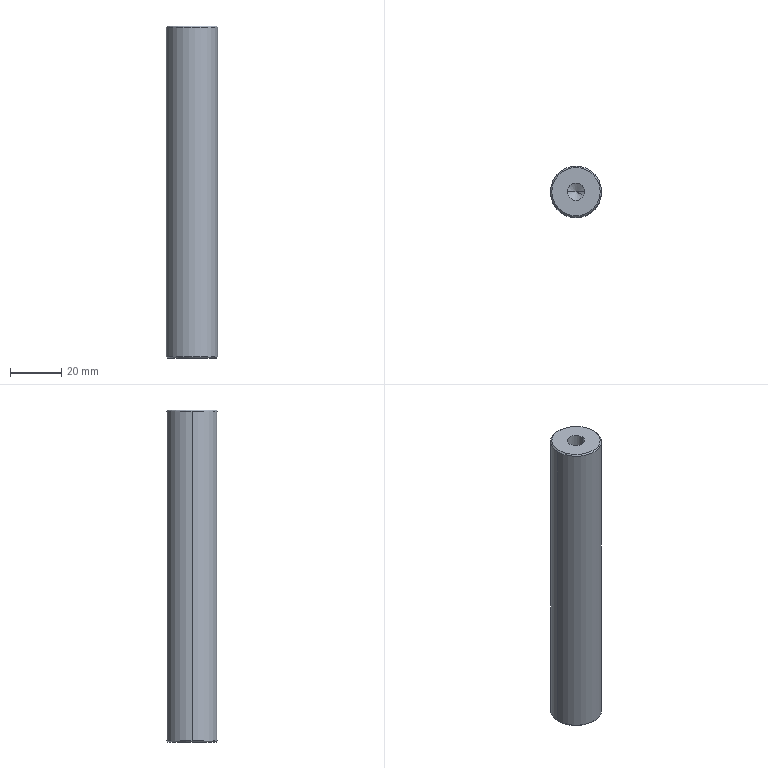Part | SolidWorks | features HoleWzd 2, Chamfer 1, Extrusion 1 | 1 solid | 16 faces | box 20 x 20 x 130 mm | volume 39341 mm3 | cone 8 | cylinder 6 | plane 2 | commonest cylinder face diameters 6.8 x4 20 x2
STEP:
#1=CARTESIAN_POINT('',(9.5,0.,130.));
#2=VERTEX_POINT('',#1);
#3=CARTESIAN_POINT('',(-9.5,0.,130.));
#4=VERTEX_POINT('',#3);
#5=CARTESIAN_POINT('',(0.,0.,130.));
#6=DIRECTION('',(0.,0.,1.));
#7=DIRECTION('',(1.,0.,0.));
#8=AXIS2_PLACEMENT_3D('',#5,#6,#7);
#9=CIRCLE('',#8,9.5);
#10=EDGE_CURVE('',#2,#4,#9,.T.);
#11=ORIENTED_EDGE('',*,*,#10,.F.);
#12=CARTESIAN_POINT('',(10.,0.,129.5));
#13=VERTEX_POINT('',#12);
#14=CARTESIAN_POINT('',(9.5,0.,130.));
#15=DIRECTION('',(0.7071,0.,-0.7071));
#16=VECTOR('',#15,1000.);
#17=LINE('',#14,#16);
#18=EDGE_CURVE('',#2,#13,#17,.T.);
#19=ORIENTED_EDGE('',*,*,#18,.T.);
#20=CARTESIAN_POINT('',(-10.,0.,129.5));
#21=VERTEX_POINT('',#20);
#22=CARTESIAN_POINT('',(0.,0.,129.5));
#23=DIRECTION('',(0.,0.,-1.));
#24=DIRECTION('',(1.,0.,0.));
#25=AXIS2_PLACEMENT_3D('',#22,#23,#24);
#26=CIRCLE('',#25,10.);
#27=EDGE_CURVE('',#21,#13,#26,.T.);
#28=ORIENTED_EDGE('',*,*,#27,.F.);
#29=CARTESIAN_POINT('',(-9.5,0.,130.));
#30=DIRECTION('',(-0.7071,0.,-0.7071));
#31=VECTOR('',#30,1000.);
#32=LINE('',#29,#31);
#33=EDGE_CURVE('',#4,#21,#32,.T.);
#34=ORIENTED_EDGE('',*,*,#33,.F.);
#35=EDGE_LOOP('',(#11,#19,#28,#34));
#36=FACE_OUTER_BOUND('',#35,.T.);
#37=CARTESIAN_POINT('',(0.,0.,130.));
#38=DIRECTION('',(0.,0.,-1.));
#39=DIRECTION('',(-1.,0.,0.));
#40=AXIS2_PLACEMENT_3D('',#37,#38,#39);
#41=CONICAL_SURFACE('',#40,9.5,0.7854);
#42=ADVANCED_FACE('',(#36),#41,.T.);
#43=CARTESIAN_POINT('',(-9.5,0.,0.));
#44=VERTEX_POINT('',#43);
#45=CARTESIAN_POINT('',(9.5,0.,0.));
#46=VERTEX_POINT('',#45);
#47=CARTESIAN_POINT('',(0.,0.,0.));
#48=DIRECTION('',(0.,0.,-1.));
#49=DIRECTION('',(1.,0.,0.));
#50=AXIS2_PLACEMENT_3D('',#47,#48,#49);
#51=CIRCLE('',#50,9.5);
#52=EDGE_CURVE('',#44,#46,#51,.T.);
#53=ORIENTED_EDGE('',*,*,#52,.F.);
#54=CARTESIAN_POINT('',(-10.,0.,0.5));
#55=VERTEX_POINT('',#54);
#56=CARTESIAN_POINT('',(-10.,0.,0.5));
#57=DIRECTION('',(-0.7071,0.,0.7071));
#58=VECTOR('',#57,1000.);
#59=LINE('',#56,#58);
#60=EDGE_CURVE('',#44,#55,#59,.T.);
#61=ORIENTED_EDGE('',*,*,#60,.T.);
#62=CARTESIAN_POINT('',(10.,0.,0.5));
#63=VERTEX_POINT('',#62);
#64=CARTESIAN_POINT('',(0.,0.,0.5));
#65=DIRECTION('',(0.,0.,1.));
#66=DIRECTION('',(1.,0.,0.));
#67=AXIS2_PLACEMENT_3D('',#64,#65,#66);
#68=CIRCLE('',#67,10.);
#69=EDGE_CURVE('',#63,#55,#68,.T.);
#70=ORIENTED_EDGE('',*,*,#69,.F.);
#71=CARTESIAN_POINT('',(10.,0.,0.5));
#72=DIRECTION('',(0.7071,0.,0.7071));
#73=VECTOR('',#72,1000.);
#74=LINE('',#71,#73);
#75=EDGE_CURVE('',#46,#63,#74,.T.);
#76=ORIENTED_EDGE('',*,*,#75,.F.);
#77=EDGE_LOOP('',(#53,#61,#70,#76));
#78=FACE_OUTER_BOUND('',#77,.T.);
#79=CARTESIAN_POINT('',(0.,0.,0.5));
#80=DIRECTION('',(0.,0.,1.));
#81=DIRECTION('',(1.,0.,0.));
#82=AXIS2_PLACEMENT_3D('',#79,#80,#81);
#83=CONICAL_SURFACE('',#82,10.,0.7854);
#84=ADVANCED_FACE('',(#78),#83,.T.);
#85=CARTESIAN_POINT('',(-3.4,0.,110.25));
#86=VERTEX_POINT('',#85);
#87=CARTESIAN_POINT('',(3.4,0.,110.25));
#88=VERTEX_POINT('',#87);
#89=CARTESIAN_POINT('',(0.,0.,110.25));
#90=DIRECTION('',(0.,0.,1.));
#91=DIRECTION('',(1.,0.,0.));
#92=AXIS2_PLACEMENT_3D('',#89,#90,#91);
#93=CIRCLE('',#92,3.4);
#94=EDGE_CURVE('',#86,#88,#93,.T.);
#95=ORIENTED_EDGE('',*,*,#94,.F.);
#96=CARTESIAN_POINT('',(-3.4,0.,130.));
#97=VERTEX_POINT('',#96);
#98=CARTESIAN_POINT('',(-3.4,0.,130.));
#99=DIRECTION('',(0.,0.,1.));
#100=VECTOR('',#99,1000.);
#101=LINE('',#98,#100);
#102=EDGE_CURVE('',#86,#97,#101,.T.);
#103=ORIENTED_EDGE('',*,*,#102,.T.);
#104=CARTESIAN_POINT('',(3.4,0.,130.));
#105=VERTEX_POINT('',#104);
#106=CARTESIAN_POINT('',(0.,0.,130.));
#107=DIRECTION('',(0.,0.,1.));
#108=DIRECTION('',(1.,0.,0.));
#109=AXIS2_PLACEMENT_3D('',#106,#107,#108);
#110=CIRCLE('',#109,3.4);
#111=EDGE_CURVE('',#97,#105,#110,.T.);
#112=ORIENTED_EDGE('',*,*,#111,.T.);
#113=CARTESIAN_POINT('',(3.4,0.,130.));
#114=DIRECTION('',(0.,0.,1.));
#115=VECTOR('',#114,1000.);
#116=LINE('',#113,#115);
#117=EDGE_CURVE('',#88,#105,#116,.T.);
#118=ORIENTED_EDGE('',*,*,#117,.F.);
#119=EDGE_LOOP('',(#95,#103,#112,#118));
#120=FACE_OUTER_BOUND('',#119,.T.);
#121=CARTESIAN_POINT('',(0.,0.,130.));
#122=DIRECTION('',(0.,0.,1.));
#123=DIRECTION('',(1.,0.,0.));
#124=AXIS2_PLACEMENT_3D('',#121,#122,#123);
#125=CYLINDRICAL_SURFACE('',#124,3.4);
#126=ADVANCED_FACE('',(#120),#125,.F.);
#127=CARTESIAN_POINT('',(0.,0.,108.207));
#128=VERTEX_POINT('',#127);
#129=CARTESIAN_POINT('',(3.4,0.,110.25));
#130=DIRECTION('',(0.8572,0.,0.515));
#131=VECTOR('',#130,1000.);
#132=LINE('',#129,#131);
#133=EDGE_CURVE('',#128,#88,#132,.T.);
#134=ORIENTED_EDGE('',*,*,#133,.F.);
#135=CARTESIAN_POINT('',(-3.4,0.,110.25));
#136=DIRECTION('',(-0.8572,0.,0.515));
#137=VECTOR('',#136,1000.);
#138=LINE('',#135,#137);
#139=EDGE_CURVE('',#128,#86,#138,.T.);
#140=ORIENTED_EDGE('',*,*,#139,.T.);
#141=ORIENTED_EDGE('',*,*,#94,.T.);
#142=EDGE_LOOP('',(#134,#140,#141));
#143=FACE_OUTER_BOUND('',#142,.T.);
#144=CARTESIAN_POINT('',(0.,0.,110.25));
#145=DIRECTION('',(0.,0.,1.));
#146=DIRECTION('',(1.,0.,0.));
#147=AXIS2_PLACEMENT_3D('',#144,#145,#146);
#148=CONICAL_SURFACE('',#147,3.4,1.03);
#149=ADVANCED_FACE('',(#143),#148,.F.);
#150=CARTESIAN_POINT('',(3.4,0.,19.75));
#151=VERTEX_POINT('',#150);
#152=CARTESIAN_POINT('',(-3.4,0.,19.75));
#153=VERTEX_POINT('',#152);
#154=CARTESIAN_POINT('',(0.,0.,19.75));
#155=DIRECTION('',(0.,0.,-1.));
#156=DIRECTION('',(-1.,0.,0.));
#157=AXIS2_PLACEMENT_3D('',#154,#155,#156);
#158=CIRCLE('',#157,3.4);
#159=EDGE_CURVE('',#151,#153,#158,.T.);
#160=ORIENTED_EDGE('',*,*,#159,.F.);
#161=CARTESIAN_POINT('',(3.4,0.,0.));
#162=VERTEX_POINT('',#161);
#163=CARTESIAN_POINT('',(3.4,0.,0.));
#164=DIRECTION('',(0.,0.,-1.));
#165=VECTOR('',#164,1000.);
#166=LINE('',#163,#165);
#167=EDGE_CURVE('',#151,#162,#166,.T.);
#168=ORIENTED_EDGE('',*,*,#167,.T.);
#169=CARTESIAN_POINT('',(-3.4,0.,0.));
#170=VERTEX_POINT('',#169);
#171=CARTESIAN_POINT('',(0.,0.,0.));
#172=DIRECTION('',(0.,0.,-1.));
#173=DIRECTION('',(-1.,0.,0.));
#174=AXIS2_PLACEMENT_3D('',#171,#172,#173);
#175=CIRCLE('',#174,3.4);
#176=EDGE_CURVE('',#162,#170,#175,.T.);
#177=ORIENTED_EDGE('',*,*,#176,.T.);
#178=CARTESIAN_POINT('',(-3.4,0.,0.));
#179=DIRECTION('',(0.,0.,-1.));
#180=VECTOR('',#179,1000.);
#181=LINE('',#178,#180);
#182=EDGE_CURVE('',#153,#170,#181,.T.);
#183=ORIENTED_EDGE('',*,*,#182,.F.);
#184=EDGE_LOOP('',(#160,#168,#177,#183));
#185=FACE_OUTER_BOUND('',#184,.T.);
#186=CARTESIAN_POINT('',(0.,0.,0.));
#187=DIRECTION('',(0.,0.,-1.));
#188=DIRECTION('',(-1.,0.,0.));
#189=AXIS2_PLACEMENT_3D('',#186,#187,#188);
#190=CYLINDRICAL_SURFACE('',#189,3.4);
#191=ADVANCED_FACE('',(#185),#190,.F.);
#192=CARTESIAN_POINT('',(0.,0.,21.793));
#193=VERTEX_POINT('',#192);
#194=CARTESIAN_POINT('',(-3.4,0.,19.75));
#195=DIRECTION('',(-0.8572,0.,-0.515));
#196=VECTOR('',#195,1000.);
#197=LINE('',#194,#196);
#198=EDGE_CURVE('',#193,#153,#197,.T.);
#199=ORIENTED_EDGE('',*,*,#198,.F.);
#200=CARTESIAN_POINT('',(3.4,0.,19.75));
#201=DIRECTION('',(0.8572,0.,-0.515));
#202=VECTOR('',#201,1000.);
#203=LINE('',#200,#202);
#204=EDGE_CURVE('',#193,#151,#203,.T.);
#205=ORIENTED_EDGE('',*,*,#204,.T.);
#206=ORIENTED_EDGE('',*,*,#159,.T.);
#207=EDGE_LOOP('',(#199,#205,#206));
#208=FACE_OUTER_BOUND('',#207,.T.);
#209=CARTESIAN_POINT('',(0.,0.,19.75));
#210=DIRECTION('',(0.,0.,-1.));
#211=DIRECTION('',(-1.,0.,0.));
#212=AXIS2_PLACEMENT_3D('',#209,#210,#211);
#213=CONICAL_SURFACE('',#212,3.4,1.03);
#214=ADVANCED_FACE('',(#208),#213,.F.);
#215=ORIENTED_EDGE('',*,*,#27,.T.);
#216=CARTESIAN_POINT('',(10.,0.,130.));
#217=DIRECTION('',(0.,0.,-1.));
#218=VECTOR('',#217,1000.);
#219=LINE('',#216,#218);
#220=EDGE_CURVE('',#13,#63,#219,.T.);
#221=ORIENTED_EDGE('',*,*,#220,.T.);
#222=ORIENTED_EDGE('',*,*,#69,.T.);
#223=CARTESIAN_POINT('',(-10.,0.,130.));
#224=DIRECTION('',(0.,0.,-1.));
#225=VECTOR('',#224,1000.);
#226=LINE('',#223,#225);
#227=EDGE_CURVE('',#21,#55,#226,.T.);
#228=ORIENTED_EDGE('',*,*,#227,.F.);
#229=EDGE_LOOP('',(#215,#221,#222,#228));
#230=FACE_OUTER_BOUND('',#229,.T.);
#231=CARTESIAN_POINT('',(0.,0.,130.));
#232=DIRECTION('',(0.,0.,-1.));
#233=DIRECTION('',(-1.,0.,0.));
#234=AXIS2_PLACEMENT_3D('',#231,#232,#233);
#235=CYLINDRICAL_SURFACE('',#234,10.);
#236=ADVANCED_FACE('',(#230),#235,.T.);
#237=ORIENTED_EDGE('',*,*,#220,.F.);
#238=CARTESIAN_POINT('',(0.,0.,129.5));
#239=DIRECTION('',(0.,0.,-1.));
#240=DIRECTION('',(1.,0.,0.));
#241=AXIS2_PLACEMENT_3D('',#238,#239,#240);
#242=CIRCLE('',#241,10.);
#243=EDGE_CURVE('',#13,#21,#242,.T.);
#244=ORIENTED_EDGE('',*,*,#243,.T.);
#245=ORIENTED_EDGE('',*,*,#227,.T.);
#246=CARTESIAN_POINT('',(0.,0.,0.5));
#247=DIRECTION('',(0.,0.,1.));
#248=DIRECTION('',(1.,0.,0.));
#249=AXIS2_PLACEMENT_3D('',#246,#247,#248);
#250=CIRCLE('',#249,10.);
#251=EDGE_CURVE('',#55,#63,#250,.T.);
#252=ORIENTED_EDGE('',*,*,#251,.T.);
#253=EDGE_LOOP('',(#237,#244,#245,#252));
#254=FACE_OUTER_BOUND('',#253,.T.);
#255=CARTESIAN_POINT('',(0.,0.,130.));
#256=DIRECTION('',(0.,0.,-1.));
#257=DIRECTION('',(-1.,0.,0.));
#258=AXIS2_PLACEMENT_3D('',#255,#256,#257);
#259=CYLINDRICAL_SURFACE('',#258,10.);
#260=ADVANCED_FACE('',(#254),#259,.T.);
#261=CARTESIAN_POINT('',(0.,0.,130.));
#262=DIRECTION('',(0.,0.,1.));
#263=DIRECTION('',(1.,0.,0.));
#264=AXIS2_PLACEMENT_3D('',#261,#262,#263);
#265=CIRCLE('',#264,9.5);
#266=EDGE_CURVE('',#4,#2,#265,.T.);
#267=ORIENTED_EDGE('',*,*,#266,.T.);
#268=ORIENTED_EDGE('',*,*,#10,.T.);
#269=EDGE_LOOP('',(#267,#268));
#270=FACE_OUTER_BOUND('',#269,.T.);
#271=CARTESIAN_POINT('',(0.,0.,130.));
#272=DIRECTION('',(0.,0.,1.));
#273=DIRECTION('',(1.,0.,0.));
#274=AXIS2_PLACEMENT_3D('',#271,#272,#273);
#275=CIRCLE('',#274,3.4);
#276=EDGE_CURVE('',#105,#97,#275,.T.);
#277=ORIENTED_EDGE('',*,*,#276,.F.);
#278=ORIENTED_EDGE('',*,*,#111,.F.);
#279=EDGE_LOOP('',(#277,#278));
#280=FACE_BOUND('',#279,.T.);
#281=CARTESIAN_POINT('',(0.,0.,130.));
#282=DIRECTION('',(0.,0.,1.));
#283=DIRECTION('',(1.,0.,0.));
#284=AXIS2_PLACEMENT_3D('',#281,#282,#283);
#285=PLANE('',#284);
#286=ADVANCED_FACE('',(#270,#280),#285,.T.);
#287=CARTESIAN_POINT('',(0.,0.,0.));
#288=DIRECTION('',(0.,0.,-1.));
#289=DIRECTION('',(1.,0.,0.));
#290=AXIS2_PLACEMENT_3D('',#287,#288,#289);
#291=CIRCLE('',#290,9.5);
#292=EDGE_CURVE('',#46,#44,#291,.T.);
#293=ORIENTED_EDGE('',*,*,#292,.T.);
#294=ORIENTED_EDGE('',*,*,#52,.T.);
#295=EDGE_LOOP('',(#293,#294));
#296=FACE_OUTER_BOUND('',#295,.T.);
#297=CARTESIAN_POINT('',(0.,0.,0.));
#298=DIRECTION('',(0.,0.,-1.));
#299=DIRECTION('',(-1.,0.,0.));
#300=AXIS2_PLACEMENT_3D('',#297,#298,#299);
#301=CIRCLE('',#300,3.4);
#302=EDGE_CURVE('',#170,#162,#301,.T.);
#303=ORIENTED_EDGE('',*,*,#302,.F.);
#304=ORIENTED_EDGE('',*,*,#176,.F.);
#305=EDGE_LOOP('',(#303,#304));
#306=FACE_BOUND('',#305,.T.);
#307=CARTESIAN_POINT('',(0.,0.,0.));
#308=DIRECTION('',(0.,0.,1.));
#309=DIRECTION('',(1.,0.,0.));
#310=AXIS2_PLACEMENT_3D('',#307,#308,#309);
#311=PLANE('',#310);
#312=ADVANCED_FACE('',(#296,#306),#311,.F.);
#313=ORIENTED_EDGE('',*,*,#204,.F.);
#314=ORIENTED_EDGE('',*,*,#198,.T.);
#315=CARTESIAN_POINT('',(0.,0.,19.75));
#316=DIRECTION('',(0.,0.,-1.));
#317=DIRECTION('',(-1.,0.,0.));
#318=AXIS2_PLACEMENT_3D('',#315,#316,#317);
#319=CIRCLE('',#318,3.4);
#320=EDGE_CURVE('',#153,#151,#319,.T.);
#321=ORIENTED_EDGE('',*,*,#320,.T.);
#322=EDGE_LOOP('',(#313,#314,#321));
#323=FACE_OUTER_BOUND('',#322,.T.);
#324=CARTESIAN_POINT('',(0.,0.,19.75));
#325=DIRECTION('',(0.,0.,-1.));
#326=DIRECTION('',(-1.,0.,0.));
#327=AXIS2_PLACEMENT_3D('',#324,#325,#326);
#328=CONICAL_SURFACE('',#327,3.4,1.03);
#329=ADVANCED_FACE('',(#323),#328,.F.);
#330=ORIENTED_EDGE('',*,*,#167,.F.);
#331=ORIENTED_EDGE('',*,*,#320,.F.);
#332=ORIENTED_EDGE('',*,*,#182,.T.);
#333=ORIENTED_EDGE('',*,*,#302,.T.);
#334=EDGE_LOOP('',(#330,#331,#332,#333));
#335=FACE_OUTER_BOUND('',#334,.T.);
#336=CARTESIAN_POINT('',(0.,0.,0.));
#337=DIRECTION('',(0.,0.,-1.));
#338=DIRECTION('',(-1.,0.,0.));
#339=AXIS2_PLACEMENT_3D('',#336,#337,#338);
#340=CYLINDRICAL_SURFACE('',#339,3.4);
#341=ADVANCED_FACE('',(#335),#340,.F.);
#342=ORIENTED_EDGE('',*,*,#139,.F.);
#343=ORIENTED_EDGE('',*,*,#133,.T.);
#344=CARTESIAN_POINT('',(0.,0.,110.25));
#345=DIRECTION('',(0.,0.,1.));
#346=DIRECTION('',(1.,0.,0.));
#347=AXIS2_PLACEMENT_3D('',#344,#345,#346);
#348=CIRCLE('',#347,3.4);
#349=EDGE_CURVE('',#88,#86,#348,.T.);
#350=ORIENTED_EDGE('',*,*,#349,.T.);
#351=EDGE_LOOP('',(#342,#343,#350));
#352=FACE_OUTER_BOUND('',#351,.T.);
#353=CARTESIAN_POINT('',(0.,0.,110.25));
#354=DIRECTION('',(0.,0.,1.));
#355=DIRECTION('',(1.,0.,0.));
#356=AXIS2_PLACEMENT_3D('',#353,#354,#355);
#357=CONICAL_SURFACE('',#356,3.4,1.03);
#358=ADVANCED_FACE('',(#352),#357,.F.);
#359=ORIENTED_EDGE('',*,*,#102,.F.);
#360=ORIENTED_EDGE('',*,*,#349,.F.);
#361=ORIENTED_EDGE('',*,*,#117,.T.);
#362=ORIENTED_EDGE('',*,*,#276,.T.);
#363=EDGE_LOOP('',(#359,#360,#361,#362));
#364=FACE_OUTER_BOUND('',#363,.T.);
#365=CARTESIAN_POINT('',(0.,0.,130.));
#366=DIRECTION('',(0.,0.,1.));
#367=DIRECTION('',(1.,0.,0.));
#368=AXIS2_PLACEMENT_3D('',#365,#366,#367);
#369=CYLINDRICAL_SURFACE('',#368,3.4);
#370=ADVANCED_FACE('',(#364),#369,.F.);
#371=ORIENTED_EDGE('',*,*,#60,.F.);
#372=ORIENTED_EDGE('',*,*,#292,.F.);
#373=ORIENTED_EDGE('',*,*,#75,.T.);
#374=ORIENTED_EDGE('',*,*,#251,.F.);
#375=EDGE_LOOP('',(#371,#372,#373,#374));
#376=FACE_OUTER_BOUND('',#375,.T.);
#377=CARTESIAN_POINT('',(0.,0.,0.5));
#378=DIRECTION('',(0.,0.,1.));
#379=DIRECTION('',(1.,0.,0.));
#380=AXIS2_PLACEMENT_3D('',#377,#378,#379);
#381=CONICAL_SURFACE('',#380,10.,0.7854);
#382=ADVANCED_FACE('',(#376),#381,.T.);
#383=ORIENTED_EDGE('',*,*,#18,.F.);
#384=ORIENTED_EDGE('',*,*,#266,.F.);
#385=ORIENTED_EDGE('',*,*,#33,.T.);
#386=ORIENTED_EDGE('',*,*,#243,.F.);
#387=EDGE_LOOP('',(#383,#384,#385,#386));
#388=FACE_OUTER_BOUND('',#387,.T.);
#389=CARTESIAN_POINT('',(0.,0.,130.));
#390=DIRECTION('',(0.,0.,-1.));
#391=DIRECTION('',(-1.,0.,0.));
#392=AXIS2_PLACEMENT_3D('',#389,#390,#391);
#393=CONICAL_SURFACE('',#392,9.5,0.7854);
#394=ADVANCED_FACE('',(#388),#393,.T.);
#395=CLOSED_SHELL('',(#42,#84,#126,#149,#191,#214,#236,#260,#286,#312,#329,#341,#358,#370,#382,#394));
#396=MANIFOLD_SOLID_BREP('',#395);
#397=CARTESIAN_POINT('',(0.,0.,0.));
#398=DIRECTION('',(0.,0.,1.));
#399=DIRECTION('',(1.,0.,0.));
#400=AXIS2_PLACEMENT_3D('',#397,#398,#399);
#401=(LENGTH_UNIT()NAMED_UNIT(*)SI_UNIT(.MILLI.,.METRE.));
#402=UNCERTAINTY_MEASURE_WITH_UNIT(LENGTH_MEASURE(0.00001),#401,'','');
#403=(NAMED_UNIT(*)PLANE_ANGLE_UNIT()SI_UNIT($,.RADIAN.));
#404=(NAMED_UNIT(*)SI_UNIT($,.STERADIAN.)SOLID_ANGLE_UNIT());
#405=(GEOMETRIC_REPRESENTATION_CONTEXT(3)GLOBAL_UNCERTAINTY_ASSIGNED_CONTEXT((#402))GLOBAL_UNIT_ASSIGNED_CONTEXT((#401,#403,#404))REPRESENTATION_CONTEXT('',''));
#406=ADVANCED_BREP_SHAPE_REPRESENTATION('',(#396,#400),#405);